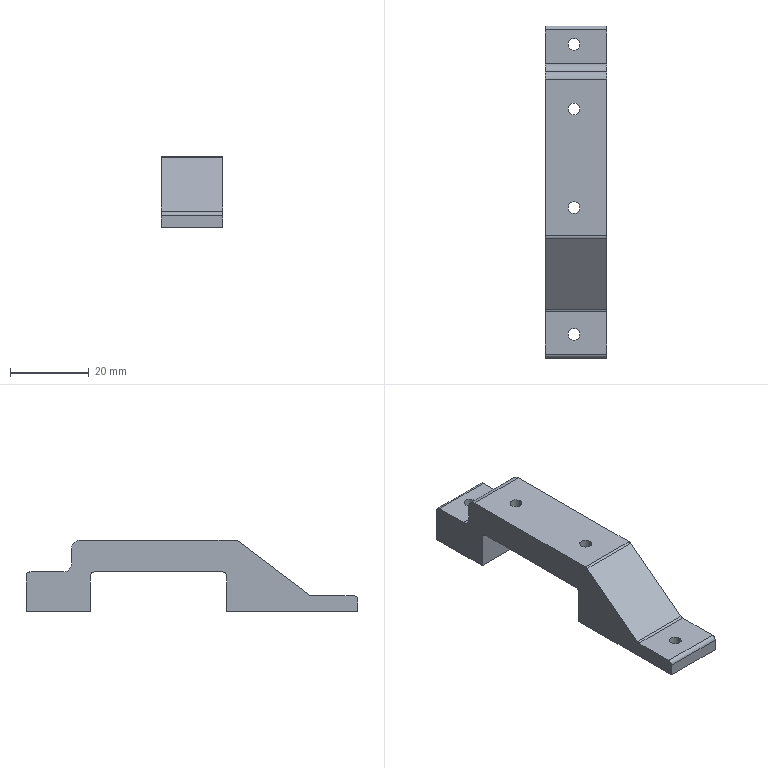Part | SolidWorks | features ICE 11, Fillet 3, Extrusion 1 | 1 solid | 30 faces | box 15.7 x 84.104 x 18.06 mm | volume 12021 mm3 | cylinder 16 | plane 14 | commonest cylinder face diameters 3 x8 2 x6 4 x2
STEP:
#1=CARTESIAN_POINT('',(-1.5,28.952,-16.06));
#2=VERTEX_POINT('',#1);
#3=CARTESIAN_POINT('',(1.5,28.952,-16.06));
#4=VERTEX_POINT('',#3);
#5=CARTESIAN_POINT('',(0.,28.952,-16.06));
#6=DIRECTION('',(0.,0.,1.));
#7=DIRECTION('',(1.,0.,0.));
#8=AXIS2_PLACEMENT_3D('',#5,#6,#7);
#9=CIRCLE('',#8,1.5);
#10=EDGE_CURVE('',#2,#4,#9,.T.);
#11=ORIENTED_EDGE('',*,*,#10,.F.);
#12=CARTESIAN_POINT('',(-1.5,28.952,-6.));
#13=VERTEX_POINT('',#12);
#14=CARTESIAN_POINT('',(-1.5,28.952,-16.06));
#15=DIRECTION('',(0.,0.,1.));
#16=VECTOR('',#15,1000.);
#17=LINE('',#14,#16);
#18=EDGE_CURVE('',#2,#13,#17,.T.);
#19=ORIENTED_EDGE('',*,*,#18,.T.);
#20=CARTESIAN_POINT('',(1.5,28.952,-6.));
#21=VERTEX_POINT('',#20);
#22=CARTESIAN_POINT('',(0.,28.952,-6.));
#23=DIRECTION('',(0.,0.,1.));
#24=DIRECTION('',(1.,0.,0.));
#25=AXIS2_PLACEMENT_3D('',#22,#23,#24);
#26=CIRCLE('',#25,1.5);
#27=EDGE_CURVE('',#13,#21,#26,.T.);
#28=ORIENTED_EDGE('',*,*,#27,.T.);
#29=CARTESIAN_POINT('',(1.5,28.952,-16.06));
#30=DIRECTION('',(0.,0.,1.));
#31=VECTOR('',#30,1000.);
#32=LINE('',#29,#31);
#33=EDGE_CURVE('',#4,#21,#32,.T.);
#34=ORIENTED_EDGE('',*,*,#33,.F.);
#35=EDGE_LOOP('',(#11,#19,#28,#34));
#36=FACE_OUTER_BOUND('',#35,.T.);
#37=CARTESIAN_POINT('',(0.,28.952,-16.06));
#38=DIRECTION('',(0.,0.,1.));
#39=DIRECTION('',(1.,0.,0.));
#40=AXIS2_PLACEMENT_3D('',#37,#38,#39);
#41=CYLINDRICAL_SURFACE('',#40,1.5);
#42=ADVANCED_FACE('',(#36),#41,.F.);
#43=CARTESIAN_POINT('',(-1.5,-44.548,-16.06));
#44=VERTEX_POINT('',#43);
#45=CARTESIAN_POINT('',(1.5,-44.548,-16.06));
#46=VERTEX_POINT('',#45);
#47=CARTESIAN_POINT('',(0.,-44.548,-16.06));
#48=DIRECTION('',(0.,0.,1.));
#49=DIRECTION('',(1.,0.,0.));
#50=AXIS2_PLACEMENT_3D('',#47,#48,#49);
#51=CIRCLE('',#50,1.5);
#52=EDGE_CURVE('',#44,#46,#51,.T.);
#53=ORIENTED_EDGE('',*,*,#52,.F.);
#54=CARTESIAN_POINT('',(-1.5,-44.548,-12.06));
#55=VERTEX_POINT('',#54);
#56=CARTESIAN_POINT('',(-1.5,-44.548,-16.06));
#57=DIRECTION('',(0.,0.,1.));
#58=VECTOR('',#57,1000.);
#59=LINE('',#56,#58);
#60=EDGE_CURVE('',#44,#55,#59,.T.);
#61=ORIENTED_EDGE('',*,*,#60,.T.);
#62=CARTESIAN_POINT('',(1.5,-44.548,-12.06));
#63=VERTEX_POINT('',#62);
#64=CARTESIAN_POINT('',(0.,-44.548,-12.06));
#65=DIRECTION('',(0.,0.,1.));
#66=DIRECTION('',(1.,0.,0.));
#67=AXIS2_PLACEMENT_3D('',#64,#65,#66);
#68=CIRCLE('',#67,1.5);
#69=EDGE_CURVE('',#55,#63,#68,.T.);
#70=ORIENTED_EDGE('',*,*,#69,.T.);
#71=CARTESIAN_POINT('',(1.5,-44.548,-16.06));
#72=DIRECTION('',(0.,0.,1.));
#73=VECTOR('',#72,1000.);
#74=LINE('',#71,#73);
#75=EDGE_CURVE('',#46,#63,#74,.T.);
#76=ORIENTED_EDGE('',*,*,#75,.F.);
#77=EDGE_LOOP('',(#53,#61,#70,#76));
#78=FACE_OUTER_BOUND('',#77,.T.);
#79=CARTESIAN_POINT('',(0.,-44.548,-16.06));
#80=DIRECTION('',(0.,0.,1.));
#81=DIRECTION('',(1.,0.,0.));
#82=AXIS2_PLACEMENT_3D('',#79,#80,#81);
#83=CYLINDRICAL_SURFACE('',#82,1.5);
#84=ADVANCED_FACE('',(#78),#83,.F.);
#85=CARTESIAN_POINT('',(-1.5,12.5,-6.));
#86=VERTEX_POINT('',#85);
#87=CARTESIAN_POINT('',(1.5,12.5,-6.));
#88=VERTEX_POINT('',#87);
#89=CARTESIAN_POINT('',(0.,12.5,-6.));
#90=DIRECTION('',(0.,0.,1.));
#91=DIRECTION('',(1.,0.,0.));
#92=AXIS2_PLACEMENT_3D('',#89,#90,#91);
#93=CIRCLE('',#92,1.5);
#94=EDGE_CURVE('',#86,#88,#93,.T.);
#95=ORIENTED_EDGE('',*,*,#94,.F.);
#96=CARTESIAN_POINT('',(-1.5,12.5,2.));
#97=VERTEX_POINT('',#96);
#98=CARTESIAN_POINT('',(-1.5,12.5,-6.));
#99=DIRECTION('',(0.,0.,1.));
#100=VECTOR('',#99,1000.);
#101=LINE('',#98,#100);
#102=EDGE_CURVE('',#86,#97,#101,.T.);
#103=ORIENTED_EDGE('',*,*,#102,.T.);
#104=CARTESIAN_POINT('',(1.5,12.5,2.));
#105=VERTEX_POINT('',#104);
#106=CARTESIAN_POINT('',(0.,12.5,2.));
#107=DIRECTION('',(0.,0.,1.));
#108=DIRECTION('',(1.,0.,0.));
#109=AXIS2_PLACEMENT_3D('',#106,#107,#108);
#110=CIRCLE('',#109,1.5);
#111=EDGE_CURVE('',#97,#105,#110,.T.);
#112=ORIENTED_EDGE('',*,*,#111,.T.);
#113=CARTESIAN_POINT('',(1.5,12.5,-6.));
#114=DIRECTION('',(0.,0.,1.));
#115=VECTOR('',#114,1000.);
#116=LINE('',#113,#115);
#117=EDGE_CURVE('',#88,#105,#116,.T.);
#118=ORIENTED_EDGE('',*,*,#117,.F.);
#119=EDGE_LOOP('',(#95,#103,#112,#118));
#120=FACE_OUTER_BOUND('',#119,.T.);
#121=CARTESIAN_POINT('',(0.,12.5,-6.));
#122=DIRECTION('',(0.,0.,1.));
#123=DIRECTION('',(1.,0.,0.));
#124=AXIS2_PLACEMENT_3D('',#121,#122,#123);
#125=CYLINDRICAL_SURFACE('',#124,1.5);
#126=ADVANCED_FACE('',(#120),#125,.F.);
#127=CARTESIAN_POINT('',(-1.5,-12.5,-6.));
#128=VERTEX_POINT('',#127);
#129=CARTESIAN_POINT('',(1.5,-12.5,-6.));
#130=VERTEX_POINT('',#129);
#131=CARTESIAN_POINT('',(0.,-12.5,-6.));
#132=DIRECTION('',(0.,0.,1.));
#133=DIRECTION('',(1.,0.,0.));
#134=AXIS2_PLACEMENT_3D('',#131,#132,#133);
#135=CIRCLE('',#134,1.5);
#136=EDGE_CURVE('',#128,#130,#135,.T.);
#137=ORIENTED_EDGE('',*,*,#136,.F.);
#138=CARTESIAN_POINT('',(-1.5,-12.5,2.));
#139=VERTEX_POINT('',#138);
#140=CARTESIAN_POINT('',(-1.5,-12.5,-6.));
#141=DIRECTION('',(0.,0.,1.));
#142=VECTOR('',#141,1000.);
#143=LINE('',#140,#142);
#144=EDGE_CURVE('',#128,#139,#143,.T.);
#145=ORIENTED_EDGE('',*,*,#144,.T.);
#146=CARTESIAN_POINT('',(1.5,-12.5,2.));
#147=VERTEX_POINT('',#146);
#148=CARTESIAN_POINT('',(0.,-12.5,2.));
#149=DIRECTION('',(0.,0.,1.));
#150=DIRECTION('',(1.,0.,0.));
#151=AXIS2_PLACEMENT_3D('',#148,#149,#150);
#152=CIRCLE('',#151,1.5);
#153=EDGE_CURVE('',#139,#147,#152,.T.);
#154=ORIENTED_EDGE('',*,*,#153,.T.);
#155=CARTESIAN_POINT('',(1.5,-12.5,-6.));
#156=DIRECTION('',(0.,0.,1.));
#157=VECTOR('',#156,1000.);
#158=LINE('',#155,#157);
#159=EDGE_CURVE('',#130,#147,#158,.T.);
#160=ORIENTED_EDGE('',*,*,#159,.F.);
#161=EDGE_LOOP('',(#137,#145,#154,#160));
#162=FACE_OUTER_BOUND('',#161,.T.);
#163=CARTESIAN_POINT('',(0.,-12.5,-6.));
#164=DIRECTION('',(0.,0.,1.));
#165=DIRECTION('',(1.,0.,0.));
#166=AXIS2_PLACEMENT_3D('',#163,#164,#165);
#167=CYLINDRICAL_SURFACE('',#166,1.5);
#168=ADVANCED_FACE('',(#162),#167,.F.);
#169=CARTESIAN_POINT('',(0.,12.5,-6.));
#170=DIRECTION('',(0.,0.,1.));
#171=DIRECTION('',(1.,0.,0.));
#172=AXIS2_PLACEMENT_3D('',#169,#170,#171);
#173=CIRCLE('',#172,1.5);
#174=EDGE_CURVE('',#88,#86,#173,.T.);
#175=ORIENTED_EDGE('',*,*,#174,.T.);
#176=ORIENTED_EDGE('',*,*,#94,.T.);
#177=EDGE_LOOP('',(#175,#176));
#178=FACE_BOUND('',#177,.T.);
#179=CARTESIAN_POINT('',(0.,-12.5,-6.));
#180=DIRECTION('',(0.,0.,1.));
#181=DIRECTION('',(1.,0.,0.));
#182=AXIS2_PLACEMENT_3D('',#179,#180,#181);
#183=CIRCLE('',#182,1.5);
#184=EDGE_CURVE('',#130,#128,#183,.T.);
#185=ORIENTED_EDGE('',*,*,#184,.T.);
#186=ORIENTED_EDGE('',*,*,#136,.T.);
#187=EDGE_LOOP('',(#185,#186));
#188=FACE_BOUND('',#187,.T.);
#189=CARTESIAN_POINT('',(8.35,16.301,-6.));
#190=VERTEX_POINT('',#189);
#191=CARTESIAN_POINT('',(8.35,-16.301,-6.));
#192=VERTEX_POINT('',#191);
#193=CARTESIAN_POINT('',(8.35,20.,-6.));
#194=DIRECTION('',(0.,-1.,0.));
#195=VECTOR('',#194,1000.);
#196=LINE('',#193,#195);
#197=EDGE_CURVE('',#190,#192,#196,.T.);
#198=ORIENTED_EDGE('',*,*,#197,.T.);
#199=CARTESIAN_POINT('',(-7.35,-16.301,-6.));
#200=VERTEX_POINT('',#199);
#201=CARTESIAN_POINT('',(0.,-16.301,-6.));
#202=DIRECTION('',(-1.,0.,0.));
#203=VECTOR('',#202,1000.);
#204=LINE('',#201,#203);
#205=EDGE_CURVE('',#192,#200,#204,.T.);
#206=ORIENTED_EDGE('',*,*,#205,.T.);
#207=CARTESIAN_POINT('',(-7.35,16.301,-6.));
#208=VERTEX_POINT('',#207);
#209=CARTESIAN_POINT('',(-7.35,17.301,-6.));
#210=DIRECTION('',(0.,-1.,0.));
#211=VECTOR('',#210,1000.);
#212=LINE('',#209,#211);
#213=EDGE_CURVE('',#208,#200,#212,.T.);
#214=ORIENTED_EDGE('',*,*,#213,.F.);
#215=CARTESIAN_POINT('',(0.,16.301,-6.));
#216=DIRECTION('',(1.,0.,0.));
#217=VECTOR('',#216,1000.);
#218=LINE('',#215,#217);
#219=EDGE_CURVE('',#208,#190,#218,.T.);
#220=ORIENTED_EDGE('',*,*,#219,.T.);
#221=EDGE_LOOP('',(#198,#206,#214,#220));
#222=FACE_OUTER_BOUND('',#221,.T.);
#223=CARTESIAN_POINT('',(0.,0.,-6.));
#224=DIRECTION('',(0.,0.,-1.));
#225=DIRECTION('',(-1.,0.,0.));
#226=AXIS2_PLACEMENT_3D('',#223,#224,#225);
#227=PLANE('',#226);
#228=ADVANCED_FACE('',(#178,#188,#222),#227,.T.);
#229=CARTESIAN_POINT('',(0.,12.5,2.));
#230=DIRECTION('',(0.,0.,1.));
#231=DIRECTION('',(1.,0.,0.));
#232=AXIS2_PLACEMENT_3D('',#229,#230,#231);
#233=CIRCLE('',#232,1.5);
#234=EDGE_CURVE('',#105,#97,#233,.T.);
#235=ORIENTED_EDGE('',*,*,#234,.F.);
#236=ORIENTED_EDGE('',*,*,#111,.F.);
#237=EDGE_LOOP('',(#235,#236));
#238=FACE_BOUND('',#237,.T.);
#239=CARTESIAN_POINT('',(0.,-12.5,2.));
#240=DIRECTION('',(0.,0.,1.));
#241=DIRECTION('',(1.,0.,0.));
#242=AXIS2_PLACEMENT_3D('',#239,#240,#241);
#243=CIRCLE('',#242,1.5);
#244=EDGE_CURVE('',#147,#139,#243,.T.);
#245=ORIENTED_EDGE('',*,*,#244,.F.);
#246=ORIENTED_EDGE('',*,*,#153,.F.);
#247=EDGE_LOOP('',(#245,#246));
#248=FACE_BOUND('',#247,.T.);
#249=CARTESIAN_POINT('',(-7.35,-19.664,2.));
#250=VERTEX_POINT('',#249);
#251=CARTESIAN_POINT('',(-7.35,20.,2.));
#252=VERTEX_POINT('',#251);
#253=CARTESIAN_POINT('',(-7.35,-20.,2.));
#254=DIRECTION('',(0.,1.,0.));
#255=VECTOR('',#254,1000.);
#256=LINE('',#253,#255);
#257=EDGE_CURVE('',#250,#252,#256,.T.);
#258=ORIENTED_EDGE('',*,*,#257,.F.);
#259=CARTESIAN_POINT('',(8.35,-19.664,2.));
#260=VERTEX_POINT('',#259);
#261=CARTESIAN_POINT('',(0.,-19.664,2.));
#262=DIRECTION('',(1.,0.,0.));
#263=VECTOR('',#262,1000.);
#264=LINE('',#261,#263);
#265=EDGE_CURVE('',#250,#260,#264,.T.);
#266=ORIENTED_EDGE('',*,*,#265,.T.);
#267=CARTESIAN_POINT('',(8.35,20.,2.));
#268=VERTEX_POINT('',#267);
#269=CARTESIAN_POINT('',(8.35,20.,2.));
#270=DIRECTION('',(0.,1.,0.));
#271=VECTOR('',#270,1000.);
#272=LINE('',#269,#271);
#273=EDGE_CURVE('',#260,#268,#272,.T.);
#274=ORIENTED_EDGE('',*,*,#273,.T.);
#275=CARTESIAN_POINT('',(0.,20.,2.));
#276=DIRECTION('',(-1.,0.,0.));
#277=VECTOR('',#276,1000.);
#278=LINE('',#275,#277);
#279=EDGE_CURVE('',#268,#252,#278,.T.);
#280=ORIENTED_EDGE('',*,*,#279,.T.);
#281=EDGE_LOOP('',(#258,#266,#274,#280));
#282=FACE_OUTER_BOUND('',#281,.T.);
#283=CARTESIAN_POINT('',(0.,0.,2.));
#284=DIRECTION('',(0.,0.,1.));
#285=DIRECTION('',(1.,0.,0.));
#286=AXIS2_PLACEMENT_3D('',#283,#284,#285);
#287=PLANE('',#286);
#288=ADVANCED_FACE('',(#238,#248,#282),#287,.T.);
#289=CARTESIAN_POINT('',(8.35,17.301,-16.06));
#290=VERTEX_POINT('',#289);
#291=CARTESIAN_POINT('',(8.35,17.301,-7.));
#292=VERTEX_POINT('',#291);
#293=CARTESIAN_POINT('',(8.35,17.301,-12.));
#294=DIRECTION('',(0.,0.,1.));
#295=VECTOR('',#294,1000.);
#296=LINE('',#293,#295);
#297=EDGE_CURVE('',#290,#292,#296,.T.);
#298=ORIENTED_EDGE('',*,*,#297,.T.);
#299=CARTESIAN_POINT('',(-7.35,17.301,-7.));
#300=VERTEX_POINT('',#299);
#301=CARTESIAN_POINT('',(8.35,17.301,-7.));
#302=DIRECTION('',(-1.,0.,0.));
#303=VECTOR('',#302,1000.);
#304=LINE('',#301,#303);
#305=EDGE_CURVE('',#292,#300,#304,.T.);
#306=ORIENTED_EDGE('',*,*,#305,.T.);
#307=CARTESIAN_POINT('',(-7.35,17.301,-16.06));
#308=VERTEX_POINT('',#307);
#309=CARTESIAN_POINT('',(-7.35,17.301,-16.06));
#310=DIRECTION('',(0.,0.,1.));
#311=VECTOR('',#310,1000.);
#312=LINE('',#309,#311);
#313=EDGE_CURVE('',#308,#300,#312,.T.);
#314=ORIENTED_EDGE('',*,*,#313,.F.);
#315=CARTESIAN_POINT('',(8.35,17.301,-16.06));
#316=DIRECTION('',(-1.,0.,0.));
#317=VECTOR('',#316,1000.);
#318=LINE('',#315,#317);
#319=EDGE_CURVE('',#290,#308,#318,.T.);
#320=ORIENTED_EDGE('',*,*,#319,.F.);
#321=EDGE_LOOP('',(#298,#306,#314,#320));
#322=FACE_OUTER_BOUND('',#321,.T.);
#323=CARTESIAN_POINT('',(8.35,17.301,-12.));
#324=DIRECTION('',(0.,1.,0.));
#325=DIRECTION('',(0.,0.,1.));
#326=AXIS2_PLACEMENT_3D('',#323,#324,#325);
#327=PLANE('',#326);
#328=ADVANCED_FACE('',(#322),#327,.F.);
#329=CARTESIAN_POINT('',(0.,28.952,-6.));
#330=DIRECTION('',(0.,0.,1.));
#331=DIRECTION('',(1.,0.,0.));
#332=AXIS2_PLACEMENT_3D('',#329,#330,#331);
#333=CIRCLE('',#332,1.5);
#334=EDGE_CURVE('',#21,#13,#333,.T.);
#335=ORIENTED_EDGE('',*,*,#334,.F.);
#336=ORIENTED_EDGE('',*,*,#27,.F.);
#337=EDGE_LOOP('',(#335,#336));
#338=FACE_BOUND('',#337,.T.);
#339=CARTESIAN_POINT('',(8.35,32.552,-6.));
#340=VERTEX_POINT('',#339);
#341=CARTESIAN_POINT('',(8.35,24.,-6.));
#342=VERTEX_POINT('',#341);
#343=CARTESIAN_POINT('',(8.35,17.301,-6.));
#344=DIRECTION('',(0.,-1.,0.));
#345=VECTOR('',#344,1000.);
#346=LINE('',#343,#345);
#347=EDGE_CURVE('',#340,#342,#346,.T.);
#348=ORIENTED_EDGE('',*,*,#347,.F.);
#349=CARTESIAN_POINT('',(-7.35,32.552,-6.));
#350=VERTEX_POINT('',#349);
#351=CARTESIAN_POINT('',(0.,32.552,-6.));
#352=DIRECTION('',(-1.,0.,0.));
#353=VECTOR('',#352,1000.);
#354=LINE('',#351,#353);
#355=EDGE_CURVE('',#340,#350,#354,.T.);
#356=ORIENTED_EDGE('',*,*,#355,.T.);
#357=CARTESIAN_POINT('',(-7.35,24.,-6.));
#358=VERTEX_POINT('',#357);
#359=CARTESIAN_POINT('',(-7.35,24.,-6.));
#360=DIRECTION('',(0.,1.,0.));
#361=VECTOR('',#360,1000.);
#362=LINE('',#359,#361);
#363=EDGE_CURVE('',#358,#350,#362,.T.);
#364=ORIENTED_EDGE('',*,*,#363,.F.);
#365=CARTESIAN_POINT('',(8.35,24.,-6.));
#366=DIRECTION('',(1.,0.,0.));
#367=VECTOR('',#366,1000.);
#368=LINE('',#365,#367);
#369=EDGE_CURVE('',#358,#342,#368,.T.);
#370=ORIENTED_EDGE('',*,*,#369,.T.);
#371=EDGE_LOOP('',(#348,#356,#364,#370));
#372=FACE_OUTER_BOUND('',#371,.T.);
#373=CARTESIAN_POINT('',(0.,0.,-6.));
#374=DIRECTION('',(0.,0.,1.));
#375=DIRECTION('',(1.,0.,0.));
#376=AXIS2_PLACEMENT_3D('',#373,#374,#375);
#377=PLANE('',#376);
#378=ADVANCED_FACE('',(#338,#372),#377,.T.);
#379=CARTESIAN_POINT('',(-7.35,-17.301,-7.));
#380=VERTEX_POINT('',#379);
#381=CARTESIAN_POINT('',(-7.35,-17.301,-16.06));
#382=VERTEX_POINT('',#381);
#383=CARTESIAN_POINT('',(-7.35,-17.301,-6.));
#384=DIRECTION('',(0.,0.,-1.));
#385=VECTOR('',#384,1000.);
#386=LINE('',#383,#385);
#387=EDGE_CURVE('',#380,#382,#386,.T.);
#388=ORIENTED_EDGE('',*,*,#387,.F.);
#389=CARTESIAN_POINT('',(8.35,-17.301,-7.));
#390=VERTEX_POINT('',#389);
#391=CARTESIAN_POINT('',(8.35,-17.301,-7.));
#392=DIRECTION('',(1.,0.,0.));
#393=VECTOR('',#392,1000.);
#394=LINE('',#391,#393);
#395=EDGE_CURVE('',#380,#390,#394,.T.);
#396=ORIENTED_EDGE('',*,*,#395,.T.);
#397=CARTESIAN_POINT('',(8.35,-17.301,-16.06));
#398=VERTEX_POINT('',#397);
#399=CARTESIAN_POINT('',(8.35,-17.301,-12.));
#400=DIRECTION('',(0.,0.,1.));
#401=VECTOR('',#400,1000.);
#402=LINE('',#399,#401);
#403=EDGE_CURVE('',#398,#390,#402,.T.);
#404=ORIENTED_EDGE('',*,*,#403,.F.);
#405=CARTESIAN_POINT('',(-8.35,-17.301,-16.06));
#406=DIRECTION('',(1.,0.,0.));
#407=VECTOR('',#406,1000.);
#408=LINE('',#405,#407);
#409=EDGE_CURVE('',#382,#398,#408,.T.);
#410=ORIENTED_EDGE('',*,*,#409,.F.);
#411=EDGE_LOOP('',(#388,#396,#404,#410));
#412=FACE_OUTER_BOUND('',#411,.T.);
#413=CARTESIAN_POINT('',(8.35,-17.301,-12.));
#414=DIRECTION('',(0.,-1.,0.));
#415=DIRECTION('',(0.,0.,-1.));
#416=AXIS2_PLACEMENT_3D('',#413,#414,#415);
#417=PLANE('',#416);
#418=ADVANCED_FACE('',(#412),#417,.F.);
#419=CARTESIAN_POINT('',(0.,-44.548,-16.06));
#420=DIRECTION('',(0.,0.,1.));
#421=DIRECTION('',(1.,0.,0.));
#422=AXIS2_PLACEMENT_3D('',#419,#420,#421);
#423=CIRCLE('',#422,1.5);
#424=EDGE_CURVE('',#46,#44,#423,.T.);
#425=ORIENTED_EDGE('',*,*,#424,.T.);
#426=ORIENTED_EDGE('',*,*,#52,.T.);
#427=EDGE_LOOP('',(#425,#426));
#428=FACE_BOUND('',#427,.T.);
#429=CARTESIAN_POINT('',(-7.35,-50.552,-16.06));
#430=VERTEX_POINT('',#429);
#431=CARTESIAN_POINT('',(8.35,-50.552,-16.06));
#432=VERTEX_POINT('',#431);
#433=CARTESIAN_POINT('',(-8.35,-50.552,-16.06));
#434=DIRECTION('',(1.,0.,0.));
#435=VECTOR('',#434,1000.);
#436=LINE('',#433,#435);
#437=EDGE_CURVE('',#430,#432,#436,.T.);
#438=ORIENTED_EDGE('',*,*,#437,.F.);
#439=CARTESIAN_POINT('',(-7.35,-17.301,-16.06));
#440=DIRECTION('',(0.,-1.,0.));
#441=VECTOR('',#440,1000.);
#442=LINE('',#439,#441);
#443=EDGE_CURVE('',#382,#430,#442,.T.);
#444=ORIENTED_EDGE('',*,*,#443,.F.);
#445=ORIENTED_EDGE('',*,*,#409,.T.);
#446=CARTESIAN_POINT('',(8.35,-17.301,-16.06));
#447=DIRECTION('',(0.,-1.,0.));
#448=VECTOR('',#447,1000.);
#449=LINE('',#446,#448);
#450=EDGE_CURVE('',#398,#432,#449,.T.);
#451=ORIENTED_EDGE('',*,*,#450,.T.);
#452=EDGE_LOOP('',(#438,#444,#445,#451));
#453=FACE_OUTER_BOUND('',#452,.T.);
#454=CARTESIAN_POINT('',(0.,0.,-16.06));
#455=DIRECTION('',(0.,0.,-1.));
#456=DIRECTION('',(-1.,0.,0.));
#457=AXIS2_PLACEMENT_3D('',#454,#455,#456);
#458=PLANE('',#457);
#459=ADVANCED_FACE('',(#428,#453),#458,.T.);
#460=CARTESIAN_POINT('',(0.,28.952,-16.06));
#461=DIRECTION('',(0.,0.,1.));
#462=DIRECTION('',(1.,0.,0.));
#463=AXIS2_PLACEMENT_3D('',#460,#461,#462);
#464=CIRCLE('',#463,1.5);
#465=EDGE_CURVE('',#4,#2,#464,.T.);
#466=ORIENTED_EDGE('',*,*,#465,.T.);
#467=ORIENTED_EDGE('',*,*,#10,.T.);
#468=EDGE_LOOP('',(#466,#467));
#469=FACE_BOUND('',#468,.T.);
#470=ORIENTED_EDGE('',*,*,#319,.T.);
#471=CARTESIAN_POINT('',(-7.35,33.552,-16.06));
#472=VERTEX_POINT('',#471);
#473=CARTESIAN_POINT('',(-7.35,33.552,-16.06));
#474=DIRECTION('',(0.,-1.,0.));
#475=VECTOR('',#474,1000.);
#476=LINE('',#473,#475);
#477=EDGE_CURVE('',#472,#308,#476,.T.);
#478=ORIENTED_EDGE('',*,*,#477,.F.);
#479=CARTESIAN_POINT('',(8.35,33.552,-16.06));
#480=VERTEX_POINT('',#479);
#481=CARTESIAN_POINT('',(8.35,33.552,-16.06));
#482=DIRECTION('',(-1.,0.,0.));
#483=VECTOR('',#482,1000.);
#484=LINE('',#481,#483);
#485=EDGE_CURVE('',#480,#472,#484,.T.);
#486=ORIENTED_EDGE('',*,*,#485,.F.);
#487=CARTESIAN_POINT('',(8.35,30.552,-16.06));
#488=DIRECTION('',(0.,-1.,0.));
#489=VECTOR('',#488,1000.);
#490=LINE('',#487,#489);
#491=EDGE_CURVE('',#480,#290,#490,.T.);
#492=ORIENTED_EDGE('',*,*,#491,.T.);
#493=EDGE_LOOP('',(#470,#478,#486,#492));
#494=FACE_OUTER_BOUND('',#493,.T.);
#495=CARTESIAN_POINT('',(0.,0.,-16.06));
#496=DIRECTION('',(0.,0.,-1.));
#497=DIRECTION('',(-1.,0.,0.));
#498=AXIS2_PLACEMENT_3D('',#495,#496,#497);
#499=PLANE('',#498);
#500=ADVANCED_FACE('',(#469,#494),#499,.T.);
#501=CARTESIAN_POINT('',(0.,-44.548,-12.06));
#502=DIRECTION('',(0.,0.,1.));
#503=DIRECTION('',(1.,0.,0.));
#504=AXIS2_PLACEMENT_3D('',#501,#502,#503);
#505=CIRCLE('',#504,1.5);
#506=EDGE_CURVE('',#63,#55,#505,.T.);
#507=ORIENTED_EDGE('',*,*,#506,.F.);
#508=ORIENTED_EDGE('',*,*,#69,.F.);
#509=EDGE_LOOP('',(#507,#508));
#510=FACE_BOUND('',#509,.T.);
#511=CARTESIAN_POINT('',(-7.35,-49.552,-12.06));
#512=VERTEX_POINT('',#511);
#513=CARTESIAN_POINT('',(-7.35,-38.881,-12.06));
#514=VERTEX_POINT('',#513);
#515=CARTESIAN_POINT('',(-7.35,-50.552,-12.06));
#516=DIRECTION('',(0.,1.,0.));
#517=VECTOR('',#516,1000.);
#518=LINE('',#515,#517);
#519=EDGE_CURVE('',#512,#514,#518,.T.);
#520=ORIENTED_EDGE('',*,*,#519,.F.);
#521=CARTESIAN_POINT('',(8.35,-49.552,-12.06));
#522=VERTEX_POINT('',#521);
#523=CARTESIAN_POINT('',(-8.35,-49.552,-12.06));
#524=DIRECTION('',(1.,0.,0.));
#525=VECTOR('',#524,1000.);
#526=LINE('',#523,#525);
#527=EDGE_CURVE('',#512,#522,#526,.T.);
#528=ORIENTED_EDGE('',*,*,#527,.T.);
#529=CARTESIAN_POINT('',(8.35,-38.881,-12.06));
#530=VERTEX_POINT('',#529);
#531=CARTESIAN_POINT('',(8.35,-50.552,-12.06));
#532=DIRECTION('',(0.,1.,0.));
#533=VECTOR('',#532,1000.);
#534=LINE('',#531,#533);
#535=EDGE_CURVE('',#522,#530,#534,.T.);
#536=ORIENTED_EDGE('',*,*,#535,.T.);
#537=CARTESIAN_POINT('',(-8.35,-38.881,-12.06));
#538=DIRECTION('',(-1.,0.,0.));
#539=VECTOR('',#538,1000.);
#540=LINE('',#537,#539);
#541=EDGE_CURVE('',#530,#514,#540,.T.);
#542=ORIENTED_EDGE('',*,*,#541,.T.);
#543=EDGE_LOOP('',(#520,#528,#536,#542));
#544=FACE_OUTER_BOUND('',#543,.T.);
#545=CARTESIAN_POINT('',(-8.35,-50.552,-12.06));
#546=DIRECTION('',(0.,0.,-1.));
#547=DIRECTION('',(-1.,0.,0.));
#548=AXIS2_PLACEMENT_3D('',#545,#546,#547);
#549=PLANE('',#548);
#550=ADVANCED_FACE('',(#510,#544),#549,.F.);
#551=CARTESIAN_POINT('',(8.35,-50.552,-13.06));
#552=VERTEX_POINT('',#551);
#553=CARTESIAN_POINT('',(8.35,-50.552,-16.06));
#554=DIRECTION('',(0.,0.,1.));
#555=VECTOR('',#554,1000.);
#556=LINE('',#553,#555);
#557=EDGE_CURVE('',#432,#552,#556,.T.);
#558=ORIENTED_EDGE('',*,*,#557,.T.);
#559=CARTESIAN_POINT('',(-7.35,-50.552,-13.06));
#560=VERTEX_POINT('',#559);
#561=CARTESIAN_POINT('',(0.,-50.552,-13.06));
#562=DIRECTION('',(-1.,0.,0.));
#563=VECTOR('',#562,1000.);
#564=LINE('',#561,#563);
#565=EDGE_CURVE('',#552,#560,#564,.T.);
#566=ORIENTED_EDGE('',*,*,#565,.T.);
#567=CARTESIAN_POINT('',(-7.35,-50.552,-16.06));
#568=DIRECTION('',(0.,0.,1.));
#569=VECTOR('',#568,1000.);
#570=LINE('',#567,#569);
#571=EDGE_CURVE('',#430,#560,#570,.T.);
#572=ORIENTED_EDGE('',*,*,#571,.F.);
#573=ORIENTED_EDGE('',*,*,#437,.T.);
#574=EDGE_LOOP('',(#558,#566,#572,#573));
#575=FACE_OUTER_BOUND('',#574,.T.);
#576=CARTESIAN_POINT('',(0.,-50.552,0.));
#577=DIRECTION('',(0.,1.,0.));
#578=DIRECTION('',(0.,0.,1.));
#579=AXIS2_PLACEMENT_3D('',#576,#577,#578);
#580=PLANE('',#579);
#581=ADVANCED_FACE('',(#575),#580,.F.);
#582=CARTESIAN_POINT('',(-7.35,-38.277,-11.857));
#583=VERTEX_POINT('',#582);
#584=CARTESIAN_POINT('',(-7.35,-20.268,1.797));
#585=VERTEX_POINT('',#584);
#586=CARTESIAN_POINT('',(-7.35,-38.545,-12.06));
#587=DIRECTION('',(0.,0.7969,0.6042));
#588=VECTOR('',#587,1000.);
#589=LINE('',#586,#588);
#590=EDGE_CURVE('',#583,#585,#589,.T.);
#591=ORIENTED_EDGE('',*,*,#590,.F.);
#592=CARTESIAN_POINT('',(8.35,-38.277,-11.857));
#593=VERTEX_POINT('',#592);
#594=CARTESIAN_POINT('',(-31.622,-38.277,-11.857));
#595=DIRECTION('',(1.,0.,0.));
#596=VECTOR('',#595,1000.);
#597=LINE('',#594,#596);
#598=EDGE_CURVE('',#583,#593,#597,.T.);
#599=ORIENTED_EDGE('',*,*,#598,.T.);
#600=CARTESIAN_POINT('',(8.35,-20.268,1.797));
#601=VERTEX_POINT('',#600);
#602=CARTESIAN_POINT('',(8.35,-30.552,-6.));
#603=DIRECTION('',(0.,-0.7969,-0.6042));
#604=VECTOR('',#603,1000.);
#605=LINE('',#602,#604);
#606=EDGE_CURVE('',#601,#593,#605,.T.);
#607=ORIENTED_EDGE('',*,*,#606,.F.);
#608=CARTESIAN_POINT('',(-31.622,-20.268,1.797));
#609=DIRECTION('',(-1.,0.,0.));
#610=VECTOR('',#609,1000.);
#611=LINE('',#608,#610);
#612=EDGE_CURVE('',#601,#585,#611,.T.);
#613=ORIENTED_EDGE('',*,*,#612,.T.);
#614=EDGE_LOOP('',(#591,#599,#607,#613));
#615=FACE_OUTER_BOUND('',#614,.T.);
#616=CARTESIAN_POINT('',(-31.622,-30.552,-6.));
#617=DIRECTION('',(0.,-0.6042,0.7969));
#618=DIRECTION('',(0.,-0.7969,-0.6042));
#619=AXIS2_PLACEMENT_3D('',#616,#617,#618);
#620=PLANE('',#619);
#621=ADVANCED_FACE('',(#615),#620,.T.);
#622=CARTESIAN_POINT('',(8.35,22.,-4.));
#623=VERTEX_POINT('',#622);
#624=CARTESIAN_POINT('',(-7.35,22.,-4.));
#625=VERTEX_POINT('',#624);
#626=CARTESIAN_POINT('',(-8.35,22.,-4.));
#627=DIRECTION('',(-1.,0.,0.));
#628=VECTOR('',#627,1000.);
#629=LINE('',#626,#628);
#630=EDGE_CURVE('',#623,#625,#629,.T.);
#631=ORIENTED_EDGE('',*,*,#630,.T.);
#632=CARTESIAN_POINT('',(-7.35,22.,0.));
#633=VERTEX_POINT('',#632);
#634=CARTESIAN_POINT('',(-7.35,22.,0.));
#635=DIRECTION('',(0.,0.,-1.));
#636=VECTOR('',#635,1000.);
#637=LINE('',#634,#636);
#638=EDGE_CURVE('',#633,#625,#637,.T.);
#639=ORIENTED_EDGE('',*,*,#638,.F.);
#640=CARTESIAN_POINT('',(8.35,22.,0.));
#641=VERTEX_POINT('',#640);
#642=CARTESIAN_POINT('',(0.,22.,0.));
#643=DIRECTION('',(1.,0.,0.));
#644=VECTOR('',#643,1000.);
#645=LINE('',#642,#644);
#646=EDGE_CURVE('',#633,#641,#645,.T.);
#647=ORIENTED_EDGE('',*,*,#646,.T.);
#648=CARTESIAN_POINT('',(8.35,22.,2.));
#649=DIRECTION('',(0.,0.,-1.));
#650=VECTOR('',#649,1000.);
#651=LINE('',#648,#650);
#652=EDGE_CURVE('',#641,#623,#651,.T.);
#653=ORIENTED_EDGE('',*,*,#652,.T.);
#654=EDGE_LOOP('',(#631,#639,#647,#653));
#655=FACE_OUTER_BOUND('',#654,.T.);
#656=CARTESIAN_POINT('',(0.,22.,0.));
#657=DIRECTION('',(0.,1.,0.));
#658=DIRECTION('',(0.,0.,1.));
#659=AXIS2_PLACEMENT_3D('',#656,#657,#658);
#660=PLANE('',#659);
#661=ADVANCED_FACE('',(#655),#660,.T.);
#662=ORIENTED_EDGE('',*,*,#646,.F.);
#663=CARTESIAN_POINT('',(-7.35,20.,0.));
#664=DIRECTION('',(-1.,0.,0.));
#665=DIRECTION('',(0.,0.,1.));
#666=AXIS2_PLACEMENT_3D('',#663,#664,#665);
#667=CIRCLE('',#666,2.);
#668=EDGE_CURVE('',#252,#633,#667,.T.);
#669=ORIENTED_EDGE('',*,*,#668,.F.);
#670=ORIENTED_EDGE('',*,*,#279,.F.);
#671=CARTESIAN_POINT('',(8.35,20.,0.));
#672=DIRECTION('',(1.,0.,0.));
#673=DIRECTION('',(0.,0.,1.));
#674=AXIS2_PLACEMENT_3D('',#671,#672,#673);
#675=CIRCLE('',#674,2.);
#676=EDGE_CURVE('',#641,#268,#675,.T.);
#677=ORIENTED_EDGE('',*,*,#676,.F.);
#678=EDGE_LOOP('',(#662,#669,#670,#677));
#679=FACE_OUTER_BOUND('',#678,.T.);
#680=CARTESIAN_POINT('',(0.,20.,0.));
#681=DIRECTION('',(1.,0.,0.));
#682=DIRECTION('',(0.,0.,-1.));
#683=AXIS2_PLACEMENT_3D('',#680,#681,#682);
#684=CYLINDRICAL_SURFACE('',#683,2.);
#685=ADVANCED_FACE('',(#679),#684,.T.);
#686=CARTESIAN_POINT('',(-7.35,24.,-4.));
#687=DIRECTION('',(1.,0.,0.));
#688=DIRECTION('',(0.,0.,1.));
#689=AXIS2_PLACEMENT_3D('',#686,#687,#688);
#690=CIRCLE('',#689,2.);
#691=EDGE_CURVE('',#625,#358,#690,.T.);
#692=ORIENTED_EDGE('',*,*,#691,.F.);
#693=ORIENTED_EDGE('',*,*,#630,.F.);
#694=CARTESIAN_POINT('',(8.35,24.,-4.));
#695=DIRECTION('',(-1.,0.,0.));
#696=DIRECTION('',(0.,0.,1.));
#697=AXIS2_PLACEMENT_3D('',#694,#695,#696);
#698=CIRCLE('',#697,2.);
#699=EDGE_CURVE('',#342,#623,#698,.T.);
#700=ORIENTED_EDGE('',*,*,#699,.F.);
#701=ORIENTED_EDGE('',*,*,#369,.F.);
#702=EDGE_LOOP('',(#692,#693,#700,#701));
#703=FACE_OUTER_BOUND('',#702,.T.);
#704=CARTESIAN_POINT('',(0.,24.,-4.));
#705=DIRECTION('',(1.,0.,0.));
#706=DIRECTION('',(0.,0.,-1.));
#707=AXIS2_PLACEMENT_3D('',#704,#705,#706);
#708=CYLINDRICAL_SURFACE('',#707,2.);
#709=ADVANCED_FACE('',(#703),#708,.F.);
#710=CARTESIAN_POINT('',(-7.35,33.552,-7.));
#711=VERTEX_POINT('',#710);
#712=CARTESIAN_POINT('',(-7.35,33.552,-6.));
#713=DIRECTION('',(0.,0.,-1.));
#714=VECTOR('',#713,1000.);
#715=LINE('',#712,#714);
#716=EDGE_CURVE('',#711,#472,#715,.T.);
#717=ORIENTED_EDGE('',*,*,#716,.F.);
#718=CARTESIAN_POINT('',(8.35,33.552,-7.));
#719=VERTEX_POINT('',#718);
#720=CARTESIAN_POINT('',(0.,33.552,-7.));
#721=DIRECTION('',(1.,0.,0.));
#722=VECTOR('',#721,1000.);
#723=LINE('',#720,#722);
#724=EDGE_CURVE('',#711,#719,#723,.T.);
#725=ORIENTED_EDGE('',*,*,#724,.T.);
#726=CARTESIAN_POINT('',(8.35,33.552,-6.));
#727=DIRECTION('',(0.,0.,-1.));
#728=VECTOR('',#727,1000.);
#729=LINE('',#726,#728);
#730=EDGE_CURVE('',#719,#480,#729,.T.);
#731=ORIENTED_EDGE('',*,*,#730,.T.);
#732=ORIENTED_EDGE('',*,*,#485,.T.);
#733=EDGE_LOOP('',(#717,#725,#731,#732));
#734=FACE_OUTER_BOUND('',#733,.T.);
#735=CARTESIAN_POINT('',(0.,33.552,0.));
#736=DIRECTION('',(0.,1.,0.));
#737=DIRECTION('',(0.,0.,1.));
#738=AXIS2_PLACEMENT_3D('',#735,#736,#737);
#739=PLANE('',#738);
#740=ADVANCED_FACE('',(#734),#739,.T.);
#741=ORIENTED_EDGE('',*,*,#535,.F.);
#742=CARTESIAN_POINT('',(8.35,-49.552,-13.06));
#743=DIRECTION('',(1.,0.,0.));
#744=DIRECTION('',(0.,0.,1.));
#745=AXIS2_PLACEMENT_3D('',#742,#743,#744);
#746=CIRCLE('',#745,1.);
#747=EDGE_CURVE('',#522,#552,#746,.T.);
#748=ORIENTED_EDGE('',*,*,#747,.T.);
#749=ORIENTED_EDGE('',*,*,#557,.F.);
#750=ORIENTED_EDGE('',*,*,#450,.F.);
#751=ORIENTED_EDGE('',*,*,#403,.T.);
#752=CARTESIAN_POINT('',(8.35,-16.301,-7.));
#753=DIRECTION('',(-1.,0.,0.));
#754=DIRECTION('',(0.,0.,1.));
#755=AXIS2_PLACEMENT_3D('',#752,#753,#754);
#756=CIRCLE('',#755,1.);
#757=EDGE_CURVE('',#390,#192,#756,.T.);
#758=ORIENTED_EDGE('',*,*,#757,.T.);
#759=ORIENTED_EDGE('',*,*,#197,.F.);
#760=CARTESIAN_POINT('',(8.35,16.301,-7.));
#761=DIRECTION('',(-1.,0.,0.));
#762=DIRECTION('',(0.,0.,1.));
#763=AXIS2_PLACEMENT_3D('',#760,#761,#762);
#764=CIRCLE('',#763,1.);
#765=EDGE_CURVE('',#190,#292,#764,.T.);
#766=ORIENTED_EDGE('',*,*,#765,.T.);
#767=ORIENTED_EDGE('',*,*,#297,.F.);
#768=ORIENTED_EDGE('',*,*,#491,.F.);
#769=ORIENTED_EDGE('',*,*,#730,.F.);
#770=CARTESIAN_POINT('',(8.35,32.552,-7.));
#771=DIRECTION('',(1.,0.,0.));
#772=DIRECTION('',(0.,0.,1.));
#773=AXIS2_PLACEMENT_3D('',#770,#771,#772);
#774=CIRCLE('',#773,1.);
#775=EDGE_CURVE('',#719,#340,#774,.T.);
#776=ORIENTED_EDGE('',*,*,#775,.T.);
#777=ORIENTED_EDGE('',*,*,#347,.T.);
#778=ORIENTED_EDGE('',*,*,#699,.T.);
#779=ORIENTED_EDGE('',*,*,#652,.F.);
#780=ORIENTED_EDGE('',*,*,#676,.T.);
#781=ORIENTED_EDGE('',*,*,#273,.F.);
#782=CARTESIAN_POINT('',(8.35,-19.664,1.));
#783=DIRECTION('',(1.,0.,0.));
#784=DIRECTION('',(0.,0.,1.));
#785=AXIS2_PLACEMENT_3D('',#782,#783,#784);
#786=CIRCLE('',#785,1.);
#787=EDGE_CURVE('',#260,#601,#786,.T.);
#788=ORIENTED_EDGE('',*,*,#787,.T.);
#789=ORIENTED_EDGE('',*,*,#606,.T.);
#790=CARTESIAN_POINT('',(8.35,-38.881,-11.06));
#791=DIRECTION('',(-1.,0.,0.));
#792=DIRECTION('',(0.,0.,1.));
#793=AXIS2_PLACEMENT_3D('',#790,#791,#792);
#794=CIRCLE('',#793,1.);
#795=EDGE_CURVE('',#593,#530,#794,.T.);
#796=ORIENTED_EDGE('',*,*,#795,.T.);
#797=EDGE_LOOP('',(#741,#748,#749,#750,#751,#758,#759,#766,#767,#768,#769,#776,#777,#778,#779,#780,#781,#788,#789,#796));
#798=FACE_OUTER_BOUND('',#797,.T.);
#799=CARTESIAN_POINT('',(8.35,20.,2.));
#800=DIRECTION('',(-1.,0.,0.));
#801=DIRECTION('',(0.,0.,1.));
#802=AXIS2_PLACEMENT_3D('',#799,#800,#801);
#803=PLANE('',#802);
#804=ADVANCED_FACE('',(#798),#803,.F.);
#805=ORIENTED_EDGE('',*,*,#144,.F.);
#806=ORIENTED_EDGE('',*,*,#184,.F.);
#807=ORIENTED_EDGE('',*,*,#159,.T.);
#808=ORIENTED_EDGE('',*,*,#244,.T.);
#809=EDGE_LOOP('',(#805,#806,#807,#808));
#810=FACE_OUTER_BOUND('',#809,.T.);
#811=CARTESIAN_POINT('',(0.,-12.5,-6.));
#812=DIRECTION('',(0.,0.,1.));
#813=DIRECTION('',(1.,0.,0.));
#814=AXIS2_PLACEMENT_3D('',#811,#812,#813);
#815=CYLINDRICAL_SURFACE('',#814,1.5);
#816=ADVANCED_FACE('',(#810),#815,.F.);
#817=ORIENTED_EDGE('',*,*,#102,.F.);
#818=ORIENTED_EDGE('',*,*,#174,.F.);
#819=ORIENTED_EDGE('',*,*,#117,.T.);
#820=ORIENTED_EDGE('',*,*,#234,.T.);
#821=EDGE_LOOP('',(#817,#818,#819,#820));
#822=FACE_OUTER_BOUND('',#821,.T.);
#823=CARTESIAN_POINT('',(0.,12.5,-6.));
#824=DIRECTION('',(0.,0.,1.));
#825=DIRECTION('',(1.,0.,0.));
#826=AXIS2_PLACEMENT_3D('',#823,#824,#825);
#827=CYLINDRICAL_SURFACE('',#826,1.5);
#828=ADVANCED_FACE('',(#822),#827,.F.);
#829=ORIENTED_EDGE('',*,*,#60,.F.);
#830=ORIENTED_EDGE('',*,*,#424,.F.);
#831=ORIENTED_EDGE('',*,*,#75,.T.);
#832=ORIENTED_EDGE('',*,*,#506,.T.);
#833=EDGE_LOOP('',(#829,#830,#831,#832));
#834=FACE_OUTER_BOUND('',#833,.T.);
#835=CARTESIAN_POINT('',(0.,-44.548,-16.06));
#836=DIRECTION('',(0.,0.,1.));
#837=DIRECTION('',(1.,0.,0.));
#838=AXIS2_PLACEMENT_3D('',#835,#836,#837);
#839=CYLINDRICAL_SURFACE('',#838,1.5);
#840=ADVANCED_FACE('',(#834),#839,.F.);
#841=ORIENTED_EDGE('',*,*,#18,.F.);
#842=ORIENTED_EDGE('',*,*,#465,.F.);
#843=ORIENTED_EDGE('',*,*,#33,.T.);
#844=ORIENTED_EDGE('',*,*,#334,.T.);
#845=EDGE_LOOP('',(#841,#842,#843,#844));
#846=FACE_OUTER_BOUND('',#845,.T.);
#847=CARTESIAN_POINT('',(0.,28.952,-16.06));
#848=DIRECTION('',(0.,0.,1.));
#849=DIRECTION('',(1.,0.,0.));
#850=AXIS2_PLACEMENT_3D('',#847,#848,#849);
#851=CYLINDRICAL_SURFACE('',#850,1.5);
#852=ADVANCED_FACE('',(#846),#851,.F.);
#853=ORIENTED_EDGE('',*,*,#571,.T.);
#854=CARTESIAN_POINT('',(-7.35,-49.552,-13.06));
#855=DIRECTION('',(-1.,0.,0.));
#856=DIRECTION('',(0.,0.,1.));
#857=AXIS2_PLACEMENT_3D('',#854,#855,#856);
#858=CIRCLE('',#857,1.);
#859=EDGE_CURVE('',#560,#512,#858,.T.);
#860=ORIENTED_EDGE('',*,*,#859,.T.);
#861=ORIENTED_EDGE('',*,*,#519,.T.);
#862=CARTESIAN_POINT('',(-7.35,-38.881,-11.06));
#863=DIRECTION('',(1.,0.,0.));
#864=DIRECTION('',(0.,0.,1.));
#865=AXIS2_PLACEMENT_3D('',#862,#863,#864);
#866=CIRCLE('',#865,1.);
#867=EDGE_CURVE('',#514,#583,#866,.T.);
#868=ORIENTED_EDGE('',*,*,#867,.T.);
#869=ORIENTED_EDGE('',*,*,#590,.T.);
#870=CARTESIAN_POINT('',(-7.35,-19.664,1.));
#871=DIRECTION('',(-1.,0.,0.));
#872=DIRECTION('',(0.,0.,1.));
#873=AXIS2_PLACEMENT_3D('',#870,#871,#872);
#874=CIRCLE('',#873,1.);
#875=EDGE_CURVE('',#585,#250,#874,.T.);
#876=ORIENTED_EDGE('',*,*,#875,.T.);
#877=ORIENTED_EDGE('',*,*,#257,.T.);
#878=ORIENTED_EDGE('',*,*,#668,.T.);
#879=ORIENTED_EDGE('',*,*,#638,.T.);
#880=ORIENTED_EDGE('',*,*,#691,.T.);
#881=ORIENTED_EDGE('',*,*,#363,.T.);
#882=CARTESIAN_POINT('',(-7.35,32.552,-7.));
#883=DIRECTION('',(-1.,0.,0.));
#884=DIRECTION('',(0.,0.,1.));
#885=AXIS2_PLACEMENT_3D('',#882,#883,#884);
#886=CIRCLE('',#885,1.);
#887=EDGE_CURVE('',#350,#711,#886,.T.);
#888=ORIENTED_EDGE('',*,*,#887,.T.);
#889=ORIENTED_EDGE('',*,*,#716,.T.);
#890=ORIENTED_EDGE('',*,*,#477,.T.);
#891=ORIENTED_EDGE('',*,*,#313,.T.);
#892=CARTESIAN_POINT('',(-7.35,16.301,-7.));
#893=DIRECTION('',(1.,0.,0.));
#894=DIRECTION('',(0.,0.,1.));
#895=AXIS2_PLACEMENT_3D('',#892,#893,#894);
#896=CIRCLE('',#895,1.);
#897=EDGE_CURVE('',#300,#208,#896,.T.);
#898=ORIENTED_EDGE('',*,*,#897,.T.);
#899=ORIENTED_EDGE('',*,*,#213,.T.);
#900=CARTESIAN_POINT('',(-7.35,-16.301,-7.));
#901=DIRECTION('',(1.,0.,0.));
#902=DIRECTION('',(0.,0.,1.));
#903=AXIS2_PLACEMENT_3D('',#900,#901,#902);
#904=CIRCLE('',#903,1.);
#905=EDGE_CURVE('',#200,#380,#904,.T.);
#906=ORIENTED_EDGE('',*,*,#905,.T.);
#907=ORIENTED_EDGE('',*,*,#387,.T.);
#908=ORIENTED_EDGE('',*,*,#443,.T.);
#909=EDGE_LOOP('',(#853,#860,#861,#868,#869,#876,#877,#878,#879,#880,#881,#888,#889,#890,#891,#898,#899,#906,#907,#908));
#910=FACE_OUTER_BOUND('',#909,.T.);
#911=CARTESIAN_POINT('',(-7.35,20.,0.));
#912=DIRECTION('',(-1.,0.,0.));
#913=DIRECTION('',(0.,0.,1.));
#914=AXIS2_PLACEMENT_3D('',#911,#912,#913);
#915=PLANE('',#914);
#916=ADVANCED_FACE('',(#910),#915,.T.);
#917=ORIENTED_EDGE('',*,*,#747,.F.);
#918=ORIENTED_EDGE('',*,*,#527,.F.);
#919=ORIENTED_EDGE('',*,*,#859,.F.);
#920=ORIENTED_EDGE('',*,*,#565,.F.);
#921=EDGE_LOOP('',(#917,#918,#919,#920));
#922=FACE_OUTER_BOUND('',#921,.T.);
#923=CARTESIAN_POINT('',(0.,-49.552,-13.06));
#924=DIRECTION('',(-1.,0.,0.));
#925=DIRECTION('',(0.,0.,1.));
#926=AXIS2_PLACEMENT_3D('',#923,#924,#925);
#927=CYLINDRICAL_SURFACE('',#926,1.);
#928=ADVANCED_FACE('',(#922),#927,.T.);
#929=ORIENTED_EDGE('',*,*,#887,.F.);
#930=ORIENTED_EDGE('',*,*,#355,.F.);
#931=ORIENTED_EDGE('',*,*,#775,.F.);
#932=ORIENTED_EDGE('',*,*,#724,.F.);
#933=EDGE_LOOP('',(#929,#930,#931,#932));
#934=FACE_OUTER_BOUND('',#933,.T.);
#935=CARTESIAN_POINT('',(0.,32.552,-7.));
#936=DIRECTION('',(1.,0.,0.));
#937=DIRECTION('',(0.,0.,-1.));
#938=AXIS2_PLACEMENT_3D('',#935,#936,#937);
#939=CYLINDRICAL_SURFACE('',#938,1.);
#940=ADVANCED_FACE('',(#934),#939,.T.);
#941=ORIENTED_EDGE('',*,*,#867,.F.);
#942=ORIENTED_EDGE('',*,*,#541,.F.);
#943=ORIENTED_EDGE('',*,*,#795,.F.);
#944=ORIENTED_EDGE('',*,*,#598,.F.);
#945=EDGE_LOOP('',(#941,#942,#943,#944));
#946=FACE_OUTER_BOUND('',#945,.T.);
#947=CARTESIAN_POINT('',(-31.622,-38.881,-11.06));
#948=DIRECTION('',(1.,0.,0.));
#949=DIRECTION('',(0.,0.,-1.));
#950=AXIS2_PLACEMENT_3D('',#947,#948,#949);
#951=CYLINDRICAL_SURFACE('',#950,1.);
#952=ADVANCED_FACE('',(#946),#951,.F.);
#953=ORIENTED_EDGE('',*,*,#875,.F.);
#954=ORIENTED_EDGE('',*,*,#612,.F.);
#955=ORIENTED_EDGE('',*,*,#787,.F.);
#956=ORIENTED_EDGE('',*,*,#265,.F.);
#957=EDGE_LOOP('',(#953,#954,#955,#956));
#958=FACE_OUTER_BOUND('',#957,.T.);
#959=CARTESIAN_POINT('',(0.,-19.664,1.));
#960=DIRECTION('',(1.,0.,0.));
#961=DIRECTION('',(0.,0.,-1.));
#962=AXIS2_PLACEMENT_3D('',#959,#960,#961);
#963=CYLINDRICAL_SURFACE('',#962,1.);
#964=ADVANCED_FACE('',(#958),#963,.T.);
#965=ORIENTED_EDGE('',*,*,#905,.F.);
#966=ORIENTED_EDGE('',*,*,#205,.F.);
#967=ORIENTED_EDGE('',*,*,#757,.F.);
#968=ORIENTED_EDGE('',*,*,#395,.F.);
#969=EDGE_LOOP('',(#965,#966,#967,#968));
#970=FACE_OUTER_BOUND('',#969,.T.);
#971=CARTESIAN_POINT('',(8.35,-16.301,-7.));
#972=DIRECTION('',(1.,0.,0.));
#973=DIRECTION('',(0.,0.,-1.));
#974=AXIS2_PLACEMENT_3D('',#971,#972,#973);
#975=CYLINDRICAL_SURFACE('',#974,1.);
#976=ADVANCED_FACE('',(#970),#975,.F.);
#977=ORIENTED_EDGE('',*,*,#765,.F.);
#978=ORIENTED_EDGE('',*,*,#219,.F.);
#979=ORIENTED_EDGE('',*,*,#897,.F.);
#980=ORIENTED_EDGE('',*,*,#305,.F.);
#981=EDGE_LOOP('',(#977,#978,#979,#980));
#982=FACE_OUTER_BOUND('',#981,.T.);
#983=CARTESIAN_POINT('',(8.35,16.301,-7.));
#984=DIRECTION('',(-1.,0.,0.));
#985=DIRECTION('',(0.,0.,1.));
#986=AXIS2_PLACEMENT_3D('',#983,#984,#985);
#987=CYLINDRICAL_SURFACE('',#986,1.);
#988=ADVANCED_FACE('',(#982),#987,.F.);
#989=CLOSED_SHELL('',(#42,#84,#126,#168,#228,#288,#328,#378,#418,#459,#500,#550,#581,#621,#661,#685,#709,#740,#804,#816,#828,#840,#852,#916,#928,#940,#952,#964,#976,#988));
#990=MANIFOLD_SOLID_BREP('',#989);
#991=CARTESIAN_POINT('',(0.,0.,0.));
#992=DIRECTION('',(0.,0.,1.));
#993=DIRECTION('',(1.,0.,0.));
#994=AXIS2_PLACEMENT_3D('',#991,#992,#993);
#995=(LENGTH_UNIT()NAMED_UNIT(*)SI_UNIT(.MILLI.,.METRE.));
#996=UNCERTAINTY_MEASURE_WITH_UNIT(LENGTH_MEASURE(0.00001),#995,'','');
#997=(NAMED_UNIT(*)PLANE_ANGLE_UNIT()SI_UNIT($,.RADIAN.));
#998=(NAMED_UNIT(*)SI_UNIT($,.STERADIAN.)SOLID_ANGLE_UNIT());
#999=(GEOMETRIC_REPRESENTATION_CONTEXT(3)GLOBAL_UNCERTAINTY_ASSIGNED_CONTEXT((#996))GLOBAL_UNIT_ASSIGNED_CONTEXT((#995,#997,#998))REPRESENTATION_CONTEXT('',''));
#1000=ADVANCED_BREP_SHAPE_REPRESENTATION('',(#990,#994),#999);